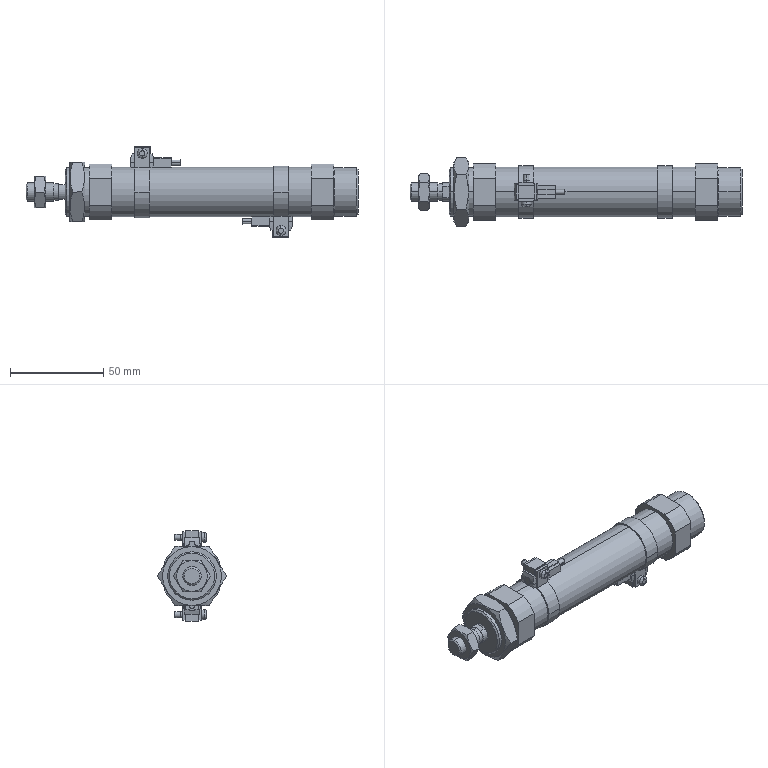Part | SolidWorks | 6 solids | 256 faces | box 178 x 36.95 x 48.66 mm | volume 71488 mm3 | plane 130 | cylinder 90 | cone 30 | spline 6 | commonest cylinder face diameters 44 x12 3 x8 26.6 x8 33.4 x8 4 x6 10 x6